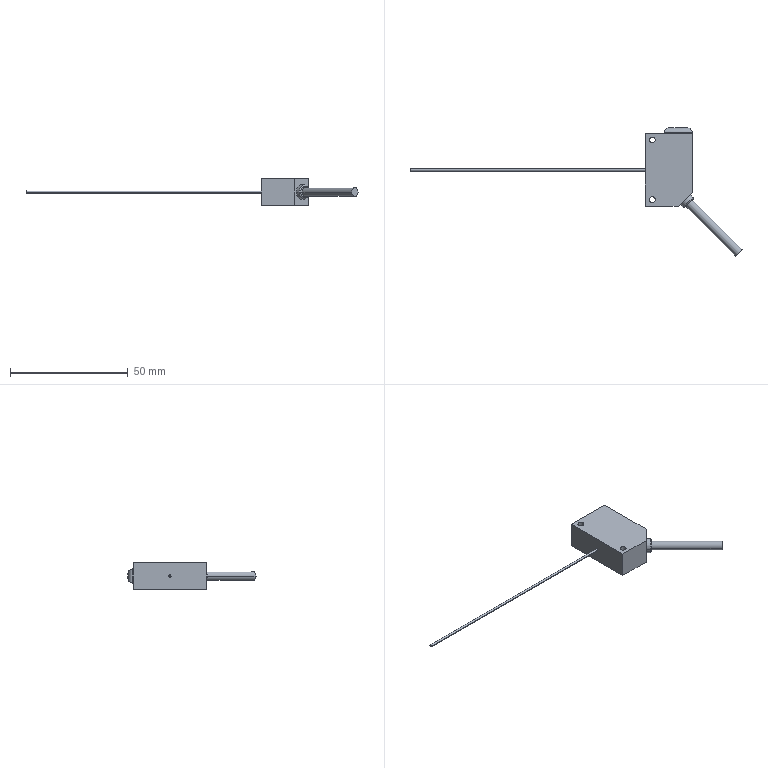Part | STEP file | Photoelectric sensor CX411D (NPN, receiver) | 1 solid | 30 faces | box 141.148 x 54.448 x 11.2 mm | volume 7234 mm3 | cylinder 14 | plane 14 | cone 2 | commonest cylinder face diameters 2.5 x4 4 x4 1 x2 3.7 x2 6 x2